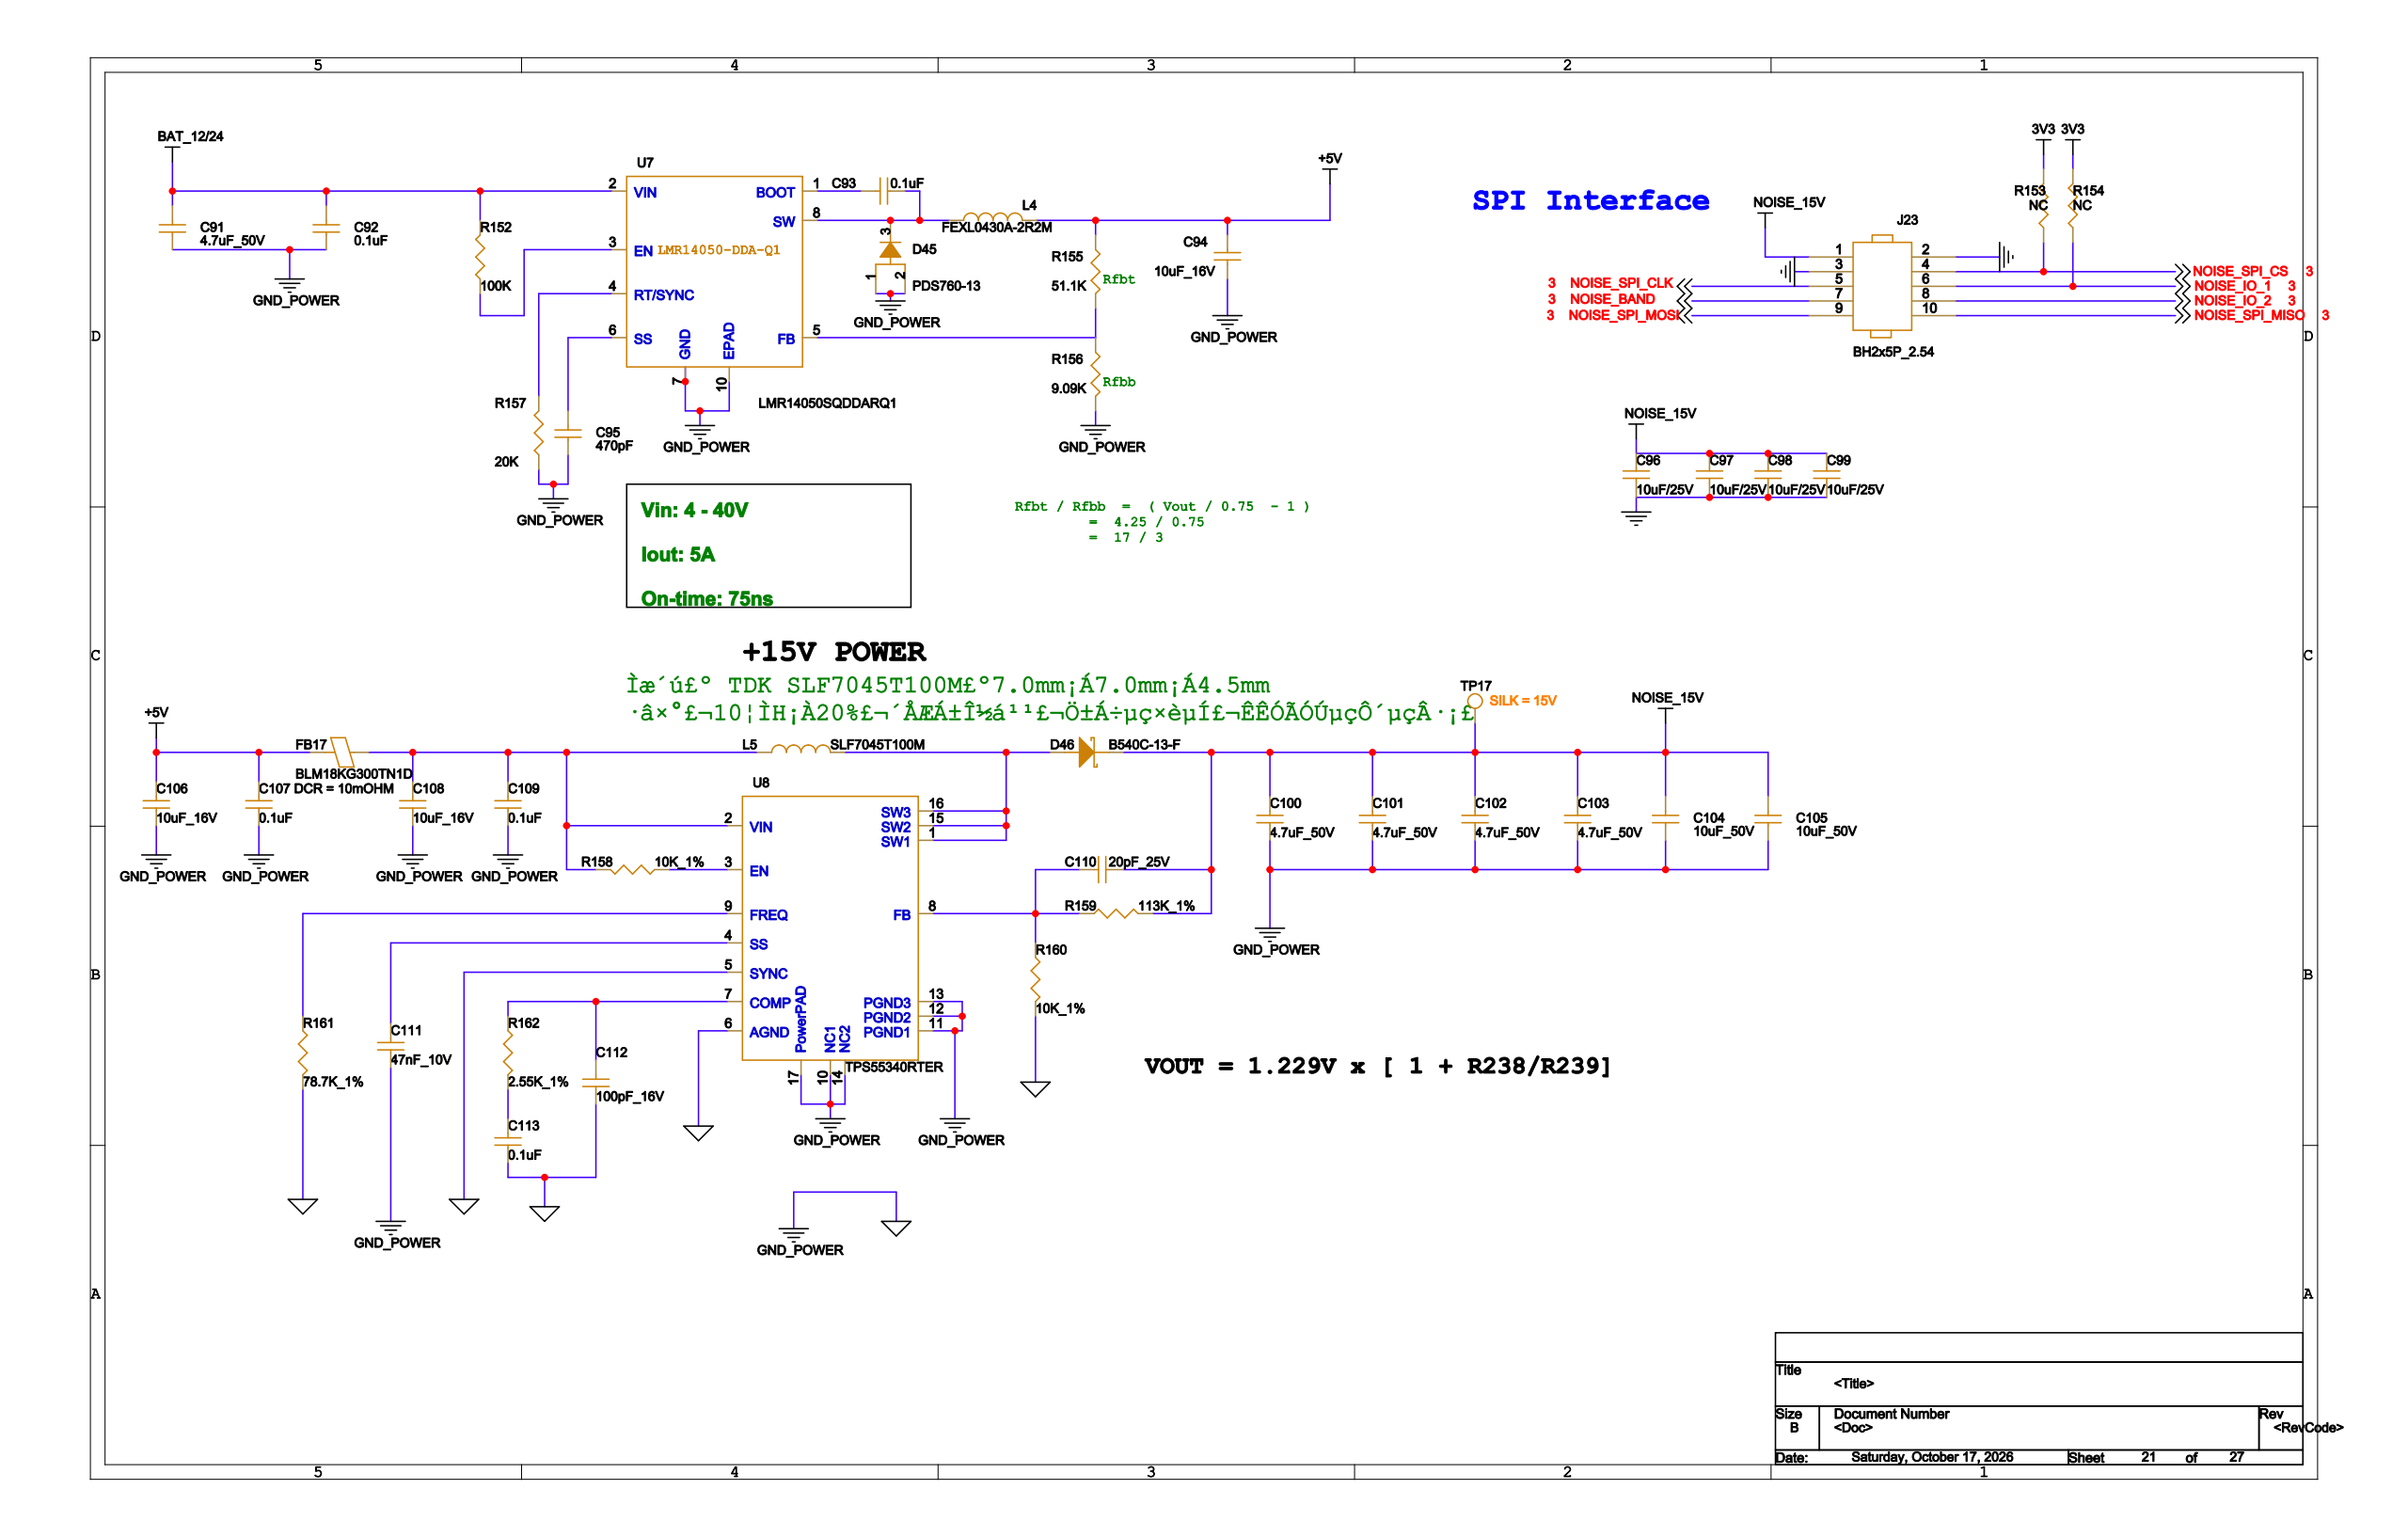Circuit board | Cadence Allegro | 477 parts | 327 nets | one sheet of the schematic
Parts on this sheet (reference | value | footprint):
C91 | 4.7uF_50V | 1206
C92 | 0.1uF | 0402
C93 | 0.1uF | 0402
C94 | 10uF_16V | 0603
C95 | 470pF | 0402
C96 | 10uF/25V | C0603
C97 | 10uF/25V | C0603
C98 | 10uF/25V | C0603
C99 | 10uF/25V | C0603
C100 | 4.7uF_50V | 1206
C101 | 4.7uF_50V | 1206
C102 | 4.7uF_50V | 1206
C103 | 4.7uF_50V | 1206
C104 | 10uF_50V | 1206
C105 | 10uF_50V | 1206
C106 | 10uF_16V | 0603
C107 | 0.1uF | 0402
C108 | 10uF_16V | 0603
C109 | 0.1uF | 0402
C110 | 20pF_25V | 0402
C111 | 47nF_10V | 0402
C112 | 100pF_16V | 0402
C113 | 0.1uF | 0402
D45 | PDS760-13 | PDS760
D46 | B540C-13-F | SMC
FB17 | BLM18KG300TN1D | 0603
J23 | BH2x5P_2.54 | BH2X5P_2_54
L4 | FEXL0430A-2R2M | L_41X41_H210_BOURNS
L5 | SLF7045T100M | SMD_7X7
R152 | 100K | 0402
R153 | NC | R0402
R154 | NC | R0402
R155 | 51.1K | 0402
R156 | 9.09K | 0402
R157 | 20K | 0402
R158 | 10K_1% | 0402
R159 | 113K_1% | 0402
R160 | 10K_1% | 0402
R161 | 78.7K_1% | 0402
R162 | 2.55K_1% | 0402
TP17 | TP | S0400CI
U7 | LMR14050SQDDARQ1 | SOP8P_60_PAD29X21_127_H170
U8 | TPS55340RTER | WQFN16-3X3
Nets of these parts (net: part-pin ...):
GND: C96-2 C97-2 C98-2 C99-2 J23-2 J23-3
BAT_GND: C91-1 C92-1 C94-2 C95-1 C100-1 C101-1 C102-1 C103-1 C104-1 C105-1 C106-1 C107-1 C108-1 C109-1 C111-1 C112-1 C113-1 D45-1 D45-2 R156-2 R157-1 R160-2 R161-2 U7-7 U7-10 U8-5 U8-6 U8-10 U8-11 U8-12 U8-13 U8-14 U8-17
3V3: R153-1 R154-1
NOISE_SPI_CS: J23-4 R153-2
NOISE_IO_1: J23-6 R154-2
BAT_12/24: C91-2 C92-2 R152-2 U7-2
NOISE_15V: C96-1 C97-1 C98-1 C99-1 C100-2 C101-2 C102-2 C103-2 C104-2 C105-2 C110-1 D46-1 J23-1 R159-2 TP17-1
N16869832: C110-2 R159-1 R160-1 U8-8
N16869875: C111-2 U8-4
N16869891: C112-2 R162-1 U8-7
N16869629: D46-2 L5-2 U8-1 U8-15 U8-16
NOISE_SPI_MISO: J23-10
NOISE_SPI_CLK: J23-5
NOISE_BAND: J23-7
NOISE_IO_2: J23-8
NOISE_SPI_MOSI: J23-9
N16869615: C108-2 C109-2 FB17-1 L5-1 R158-2 U8-2
N16869446: R152-1 U7-3
N16869473: R157-2 U7-4
N16869860: R161-1 U8-9
N16869963: C113-2 R162-2
N16869830: R158-1 U8-3
N16869365: C93-1 D45-3 L4-1 U7-8
+5V: C94-1 C106-2 C107-2 FB17-2 L4-2 R155-1
N16869493: C95-2 U7-6
N16869486: R155-2 R156-1 U7-5
N16869363: C93-2 U7-1